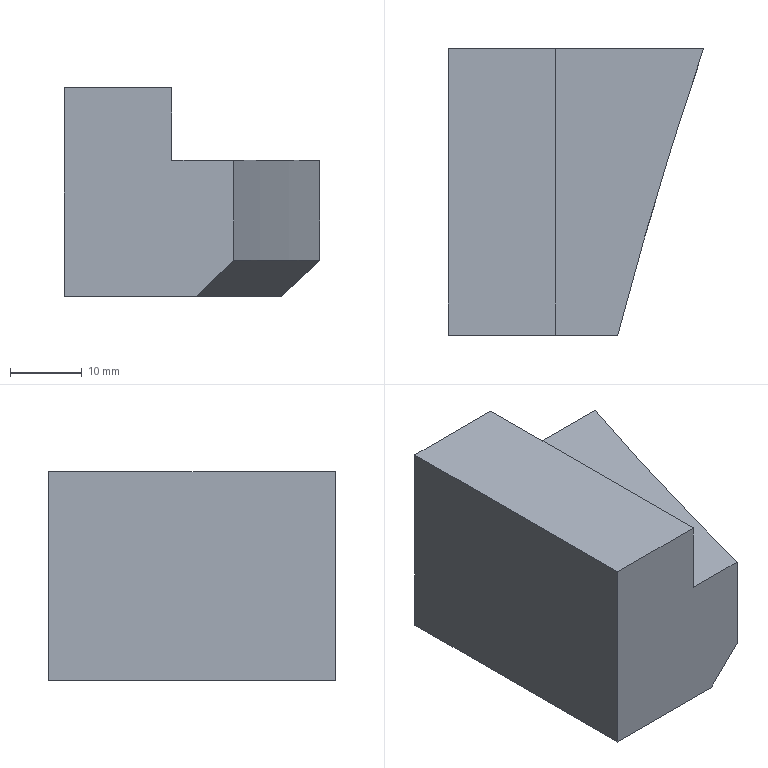Part | STEP file | Positioning_id250_x_t | 1 solid | 9 faces | box 35.628 x 40 x 29.102 mm | volume 27843 mm3 | plane 7 | spline 2
STEP:
#1=CARTESIAN_POINT('',(0.,0.,0.));
#2=DIRECTION('',(0.,0.,1.));
#3=DIRECTION('',(1.,0.,0.));
#4=AXIS2_PLACEMENT_3D('',#1,#2,#3);
#5=CARTESIAN_POINT('',(-770.37,465.,235.893));
#6=VERTEX_POINT('',#5);
#7=CARTESIAN_POINT('',(-765.202,465.,240.893));
#8=VERTEX_POINT('',#7);
#9=CARTESIAN_POINT('',(-770.37,465.,235.893));
#10=CARTESIAN_POINT('',(-769.508,465.,236.726));
#11=CARTESIAN_POINT('',(-768.647,465.,237.56));
#12=CARTESIAN_POINT('',(-767.786,465.,238.393));
#13=CARTESIAN_POINT('',(-766.924,465.,239.226));
#14=CARTESIAN_POINT('',(-766.063,465.,240.06));
#15=CARTESIAN_POINT('',(-765.202,465.,240.893));
#16=B_SPLINE_CURVE_WITH_KNOTS('',3,(#9,#10,#11,#12,#13,#14,#15),.UNSPECIFIED.,.F.,.F.,(4,3,4),(0.,0.5,1.),.UNSPECIFIED.);
#17=CARTESIAN_POINT('',(-765.482,463.728,240.943));
#18=CARTESIAN_POINT('',(-763.676,470.672,240.943));
#19=CARTESIAN_POINT('',(-759.81,484.505,240.943));
#20=CARTESIAN_POINT('',(-755.452,498.19,240.943));
#21=CARTESIAN_POINT('',(-753.154,504.984,240.943));
#22=CARTESIAN_POINT('',(-765.498,463.733,240.926));
#23=CARTESIAN_POINT('',(-763.692,470.676,240.926));
#24=CARTESIAN_POINT('',(-759.826,484.51,240.926));
#25=CARTESIAN_POINT('',(-755.468,498.195,240.926));
#26=CARTESIAN_POINT('',(-753.169,504.989,240.926));
#27=CARTESIAN_POINT('',(-765.514,463.737,240.909));
#28=CARTESIAN_POINT('',(-763.708,470.681,240.909));
#29=CARTESIAN_POINT('',(-759.842,484.515,240.909));
#30=CARTESIAN_POINT('',(-755.484,498.2,240.909));
#31=CARTESIAN_POINT('',(-753.185,504.995,240.909));
#32=CARTESIAN_POINT('',(-765.531,463.741,240.893));
#33=CARTESIAN_POINT('',(-763.724,470.685,240.893));
#34=CARTESIAN_POINT('',(-759.858,484.52,240.893));
#35=CARTESIAN_POINT('',(-755.5,498.205,240.893));
#36=CARTESIAN_POINT('',(-753.201,505.,240.893));
#37=CARTESIAN_POINT('',(-767.144,464.161,239.226));
#38=CARTESIAN_POINT('',(-765.332,471.124,239.226));
#39=CARTESIAN_POINT('',(-761.455,484.997,239.226));
#40=CARTESIAN_POINT('',(-757.085,498.72,239.226));
#41=CARTESIAN_POINT('',(-754.78,505.534,239.226));
#42=CARTESIAN_POINT('',(-768.757,464.58,237.559));
#43=CARTESIAN_POINT('',(-766.94,471.563,237.559));
#44=CARTESIAN_POINT('',(-763.052,485.474,237.559));
#45=CARTESIAN_POINT('',(-758.67,499.236,237.559));
#46=CARTESIAN_POINT('',(-756.358,506.068,237.559));
#47=CARTESIAN_POINT('',(-770.37,465.,235.893));
#48=CARTESIAN_POINT('',(-768.548,472.002,235.893));
#49=CARTESIAN_POINT('',(-764.65,485.952,235.893));
#50=CARTESIAN_POINT('',(-760.255,499.751,235.893));
#51=CARTESIAN_POINT('',(-757.937,506.602,235.893));
#52=B_SPLINE_SURFACE_WITH_KNOTS('',3,3,((#17,#18,#19,#20,#21),(#22,#23,#24,#25,#26),(#27,#28,#29,#30,#31),(#32,#33,#34,#35,#36),(#37,#38,#39,#40,#41),(#42,#43,#44,#45,#46),(#47,#48,#49,#50,#51)),.UNSPECIFIED.,.F.,.F.,.F.,(4,3,4),(4,1,4),(0.,0.009901,1.),(0.,0.5,1.),.UNSPECIFIED.);
#53=CARTESIAN_POINT('',(1.,0.));
#54=CARTESIAN_POINT('',(0.009901,0.03023));
#55=B_SPLINE_CURVE_WITH_KNOTS('',1,(#53,#54),.UNSPECIFIED.,.F.,.F.,(2,2),(0.,1.),.PIECEWISE_BEZIER_KNOTS.);
#56=(GEOMETRIC_REPRESENTATION_CONTEXT(2)PARAMETRIC_REPRESENTATION_CONTEXT()REPRESENTATION_CONTEXT('',''));
#57=DEFINITIONAL_REPRESENTATION('',(#55),#56);
#58=PCURVE('',#52,#57);
#59=CARTESIAN_POINT('',(-863.829,465.,302.856));
#60=DIRECTION('',(0.,-1.,0.));
#61=DIRECTION('',(0.,0.,1.));
#62=AXIS2_PLACEMENT_3D('',#59,#60,#61);
#63=PLANE('',#62);
#64=CARTESIAN_POINT('',(-66.963,-93.459));
#65=CARTESIAN_POINT('',(-66.13,-94.32));
#66=CARTESIAN_POINT('',(-65.296,-95.182));
#67=CARTESIAN_POINT('',(-64.463,-96.043));
#68=CARTESIAN_POINT('',(-63.63,-96.904));
#69=CARTESIAN_POINT('',(-62.796,-97.766));
#70=CARTESIAN_POINT('',(-61.963,-98.627));
#71=B_SPLINE_CURVE_WITH_KNOTS('',3,(#64,#65,#66,#67,#68,#69,#70),.UNSPECIFIED.,.F.,.F.,(4,3,4),(0.,0.5,1.),.UNSPECIFIED.);
#72=(GEOMETRIC_REPRESENTATION_CONTEXT(2)PARAMETRIC_REPRESENTATION_CONTEXT()REPRESENTATION_CONTEXT('',''));
#73=DEFINITIONAL_REPRESENTATION('',(#71),#72);
#74=PCURVE('',#63,#73);
#75=SURFACE_CURVE('',#16,(#58,#74),.PCURVE_S1.);
#76=EDGE_CURVE('',#6,#8,#75,.T.);
#77=ORIENTED_EDGE('',*,*,#76,.F.);
#78=CARTESIAN_POINT('',(-758.477,505.,235.893));
#79=VERTEX_POINT('',#78);
#80=CARTESIAN_POINT('',(-758.477,505.,235.893));
#81=CARTESIAN_POINT('',(-760.597,498.676,235.893));
#82=CARTESIAN_POINT('',(-764.802,485.408,235.893));
#83=CARTESIAN_POINT('',(-768.548,472.002,235.893));
#84=CARTESIAN_POINT('',(-770.37,465.,235.893));
#85=B_SPLINE_CURVE_WITH_KNOTS('',3,(#80,#81,#82,#83,#84),.UNSPECIFIED.,.F.,.F.,(4,1,4),(0.,0.4797,1.),.UNSPECIFIED.);
#86=CARTESIAN_POINT('',(1.,0.961));
#87=CARTESIAN_POINT('',(1.,0.));
#88=B_SPLINE_CURVE_WITH_KNOTS('',1,(#86,#87),.UNSPECIFIED.,.F.,.F.,(2,2),(0.,1.),.PIECEWISE_BEZIER_KNOTS.);
#89=(GEOMETRIC_REPRESENTATION_CONTEXT(2)PARAMETRIC_REPRESENTATION_CONTEXT()REPRESENTATION_CONTEXT('',''));
#90=DEFINITIONAL_REPRESENTATION('',(#88),#89);
#91=PCURVE('',#52,#90);
#92=CARTESIAN_POINT('',(-788.829,465.,235.893));
#93=DIRECTION('',(0.,0.,1.));
#94=DIRECTION('',(1.,0.,0.));
#95=AXIS2_PLACEMENT_3D('',#92,#93,#94);
#96=PLANE('',#95);
#97=CARTESIAN_POINT('',(30.352,40.));
#98=CARTESIAN_POINT('',(28.232,33.675));
#99=CARTESIAN_POINT('',(24.027,20.408));
#100=CARTESIAN_POINT('',(20.281,7.002));
#101=CARTESIAN_POINT('',(18.459,-0.000000011));
#102=B_SPLINE_CURVE_WITH_KNOTS('',3,(#97,#98,#99,#100,#101),.UNSPECIFIED.,.F.,.F.,(4,1,4),(0.,0.4797,1.),.UNSPECIFIED.);
#103=(GEOMETRIC_REPRESENTATION_CONTEXT(2)PARAMETRIC_REPRESENTATION_CONTEXT()REPRESENTATION_CONTEXT('',''));
#104=DEFINITIONAL_REPRESENTATION('',(#102),#103);
#105=PCURVE('',#96,#104);
#106=SURFACE_CURVE('',#85,(#91,#105),.PCURVE_S1.);
#107=EDGE_CURVE('',#79,#6,#106,.T.);
#108=ORIENTED_EDGE('',*,*,#107,.F.);
#109=CARTESIAN_POINT('',(-753.201,505.,240.893));
#110=VERTEX_POINT('',#109);
#111=CARTESIAN_POINT('',(-753.201,505.,240.893));
#112=CARTESIAN_POINT('',(-754.08,505.,240.06));
#113=CARTESIAN_POINT('',(-754.96,505.,239.226));
#114=CARTESIAN_POINT('',(-755.839,505.,238.393));
#115=CARTESIAN_POINT('',(-756.718,505.,237.56));
#116=CARTESIAN_POINT('',(-757.598,505.,236.726));
#117=CARTESIAN_POINT('',(-758.477,505.,235.893));
#118=B_SPLINE_CURVE_WITH_KNOTS('',3,(#111,#112,#113,#114,#115,#116,#117),.UNSPECIFIED.,.F.,.F.,(4,3,4),(0.,0.5,1.),.UNSPECIFIED.);
#119=CARTESIAN_POINT('',(0.009906,1.));
#120=CARTESIAN_POINT('',(1.,0.961));
#121=B_SPLINE_CURVE_WITH_KNOTS('',1,(#119,#120),.UNSPECIFIED.,.F.,.F.,(2,2),(0.,1.),.PIECEWISE_BEZIER_KNOTS.);
#122=(GEOMETRIC_REPRESENTATION_CONTEXT(2)PARAMETRIC_REPRESENTATION_CONTEXT()REPRESENTATION_CONTEXT('',''));
#123=DEFINITIONAL_REPRESENTATION('',(#121),#122);
#124=PCURVE('',#52,#123);
#125=CARTESIAN_POINT('',(-863.829,505.,302.856));
#126=DIRECTION('',(0.,1.,0.));
#127=DIRECTION('',(0.,0.,-1.));
#128=AXIS2_PLACEMENT_3D('',#125,#126,#127);
#129=PLANE('',#128);
#130=CARTESIAN_POINT('',(61.963,-110.628));
#131=CARTESIAN_POINT('',(62.796,-109.748));
#132=CARTESIAN_POINT('',(63.629,-108.869));
#133=CARTESIAN_POINT('',(64.463,-107.99));
#134=CARTESIAN_POINT('',(65.296,-107.11));
#135=CARTESIAN_POINT('',(66.13,-106.231));
#136=CARTESIAN_POINT('',(66.963,-105.352));
#137=B_SPLINE_CURVE_WITH_KNOTS('',3,(#130,#131,#132,#133,#134,#135,#136),.UNSPECIFIED.,.F.,.F.,(4,3,4),(0.,0.5,1.),.UNSPECIFIED.);
#138=(GEOMETRIC_REPRESENTATION_CONTEXT(2)PARAMETRIC_REPRESENTATION_CONTEXT()REPRESENTATION_CONTEXT('',''));
#139=DEFINITIONAL_REPRESENTATION('',(#137),#138);
#140=PCURVE('',#129,#139);
#141=SURFACE_CURVE('',#118,(#124,#140),.PCURVE_S1.);
#142=EDGE_CURVE('',#110,#79,#141,.T.);
#143=ORIENTED_EDGE('',*,*,#142,.F.);
#144=CARTESIAN_POINT('',(-765.202,465.,240.893));
#145=CARTESIAN_POINT('',(-764.004,469.56,240.893));
#146=CARTESIAN_POINT('',(-762.753,474.107,240.893));
#147=CARTESIAN_POINT('',(-761.449,478.638,240.893));
#148=CARTESIAN_POINT('',(-760.176,483.061,240.893));
#149=CARTESIAN_POINT('',(-758.852,487.47,240.893));
#150=CARTESIAN_POINT('',(-757.478,491.863,240.893));
#151=CARTESIAN_POINT('',(-756.102,496.258,240.893));
#152=CARTESIAN_POINT('',(-754.677,500.638,240.893));
#153=CARTESIAN_POINT('',(-753.201,505.,240.893));
#154=B_SPLINE_CURVE_WITH_KNOTS('',3,(#144,#145,#146,#147,#148,#149,#150,#151,#152,#153),.UNSPECIFIED.,.F.,.F.,(4,3,3,4),(0.,0.3386,0.6692,1.),.UNSPECIFIED.);
#155=CARTESIAN_POINT('',(0.009894,0.03023));
#156=CARTESIAN_POINT('',(0.009903,1.));
#157=B_SPLINE_CURVE_WITH_KNOTS('',1,(#155,#156),.UNSPECIFIED.,.F.,.F.,(2,2),(0.,1.),.PIECEWISE_BEZIER_KNOTS.);
#158=(GEOMETRIC_REPRESENTATION_CONTEXT(2)PARAMETRIC_REPRESENTATION_CONTEXT()REPRESENTATION_CONTEXT('',''));
#159=DEFINITIONAL_REPRESENTATION('',(#157),#158);
#160=PCURVE('',#52,#159);
#161=CARTESIAN_POINT('',(-753.201,505.,240.753));
#162=CARTESIAN_POINT('',(-753.201,505.,240.893));
#163=CARTESIAN_POINT('',(-753.201,505.,254.856));
#164=CARTESIAN_POINT('',(-757.663,491.811,240.753));
#165=CARTESIAN_POINT('',(-757.663,491.811,240.893));
#166=CARTESIAN_POINT('',(-757.663,491.811,254.856));
#167=CARTESIAN_POINT('',(-761.665,478.472,240.753));
#168=CARTESIAN_POINT('',(-761.665,478.472,240.893));
#169=CARTESIAN_POINT('',(-761.665,478.472,254.856));
#170=CARTESIAN_POINT('',(-765.202,465.,240.753));
#171=CARTESIAN_POINT('',(-765.202,465.,240.893));
#172=CARTESIAN_POINT('',(-765.202,465.,254.856));
#173=CARTESIAN_POINT('',(-765.237,464.865,240.753));
#174=CARTESIAN_POINT('',(-765.237,464.865,240.893));
#175=CARTESIAN_POINT('',(-765.237,464.865,254.856));
#176=CARTESIAN_POINT('',(-765.272,464.731,240.753));
#177=CARTESIAN_POINT('',(-765.272,464.731,240.893));
#178=CARTESIAN_POINT('',(-765.272,464.731,254.856));
#179=CARTESIAN_POINT('',(-765.308,464.596,240.753));
#180=CARTESIAN_POINT('',(-765.308,464.596,240.893));
#181=CARTESIAN_POINT('',(-765.308,464.596,254.856));
#182=(BOUNDED_SURFACE()B_SPLINE_SURFACE(3,1,((#161,#162,#163),(#164,#165,#166),(#167,#168,#169),(#170,#171,#172),(#173,#174,#175),(#176,#177,#178),(#179,#180,#181)),.UNSPECIFIED.,.F.,.F.,.F.)B_SPLINE_SURFACE_WITH_KNOTS((4,3,4),(2,1,2),(0.,0.9901,1.),(0.,0.009901,1.),.UNSPECIFIED.)GEOMETRIC_REPRESENTATION_ITEM()RATIONAL_B_SPLINE_SURFACE(((0.9919,0.9919,0.9919),(0.9912,0.9912,0.9912),(0.9909,0.9909,0.9909),(0.9909,0.9909,0.9909),(0.9909,0.9909,0.9909),(0.9909,0.9909,0.9909),(0.9909,0.9909,0.9909)))REPRESENTATION_ITEM('')SURFACE());
#183=CARTESIAN_POINT('',(0.9901,0.009906));
#184=CARTESIAN_POINT('',(0.,0.009903));
#185=B_SPLINE_CURVE_WITH_KNOTS('',1,(#183,#184),.UNSPECIFIED.,.F.,.F.,(2,2),(0.,1.),.PIECEWISE_BEZIER_KNOTS.);
#186=(GEOMETRIC_REPRESENTATION_CONTEXT(2)PARAMETRIC_REPRESENTATION_CONTEXT()REPRESENTATION_CONTEXT('',''));
#187=DEFINITIONAL_REPRESENTATION('',(#185),#186);
#188=PCURVE('',#182,#187);
#189=SURFACE_CURVE('',#154,(#160,#188),.PCURVE_S1.);
#190=EDGE_CURVE('',#8,#110,#189,.T.);
#191=ORIENTED_EDGE('',*,*,#190,.F.);
#192=EDGE_LOOP('',(#77,#108,#143,#191));
#193=FACE_BOUND('',#192,.T.);
#194=ADVANCED_FACE('',(#193),#52,.T.);
#195=CARTESIAN_POINT('',(-788.829,465.,235.893));
#196=VERTEX_POINT('',#195);
#197=CARTESIAN_POINT('',(-788.829,505.,235.893));
#198=VERTEX_POINT('',#197);
#199=CARTESIAN_POINT('',(-788.829,465.,235.893));
#200=DIRECTION('',(0.,1.,0.));
#201=VECTOR('',#200,1.);
#202=LINE('',#199,#201);
#203=CARTESIAN_POINT('',(0.,0.));
#204=DIRECTION('',(0.,1.));
#205=VECTOR('',#204,1.);
#206=LINE('',#203,#205);
#207=(GEOMETRIC_REPRESENTATION_CONTEXT(2)PARAMETRIC_REPRESENTATION_CONTEXT()REPRESENTATION_CONTEXT('',''));
#208=DEFINITIONAL_REPRESENTATION('',(#206),#207);
#209=PCURVE('',#96,#208);
#210=CARTESIAN_POINT('',(-788.829,493.037,302.856));
#211=DIRECTION('',(-1.,0.,0.));
#212=DIRECTION('',(0.,0.,1.));
#213=AXIS2_PLACEMENT_3D('',#210,#211,#212);
#214=PLANE('',#213);
#215=CARTESIAN_POINT('',(-66.963,-28.037));
#216=DIRECTION('',(0.,1.));
#217=VECTOR('',#216,1.);
#218=LINE('',#215,#217);
#219=(GEOMETRIC_REPRESENTATION_CONTEXT(2)PARAMETRIC_REPRESENTATION_CONTEXT()REPRESENTATION_CONTEXT('',''));
#220=DEFINITIONAL_REPRESENTATION('',(#218),#219);
#221=PCURVE('',#214,#220);
#222=SURFACE_CURVE('',#202,(#209,#221),.PCURVE_S1.);
#223=EDGE_CURVE('',#196,#198,#222,.T.);
#224=ORIENTED_EDGE('',*,*,#223,.F.);
#225=CARTESIAN_POINT('',(-770.37,465.,235.893));
#226=DIRECTION('',(-1.,0.,0.));
#227=VECTOR('',#226,1.);
#228=LINE('',#225,#227);
#229=CARTESIAN_POINT('',(18.459,0.));
#230=DIRECTION('',(-1.,0.));
#231=VECTOR('',#230,1.);
#232=LINE('',#229,#231);
#233=(GEOMETRIC_REPRESENTATION_CONTEXT(2)PARAMETRIC_REPRESENTATION_CONTEXT()REPRESENTATION_CONTEXT('',''));
#234=DEFINITIONAL_REPRESENTATION('',(#232),#233);
#235=PCURVE('',#96,#234);
#236=CARTESIAN_POINT('',(-66.963,-93.459));
#237=DIRECTION('',(0.,1.));
#238=VECTOR('',#237,1.);
#239=LINE('',#236,#238);
#240=(GEOMETRIC_REPRESENTATION_CONTEXT(2)PARAMETRIC_REPRESENTATION_CONTEXT()REPRESENTATION_CONTEXT('',''));
#241=DEFINITIONAL_REPRESENTATION('',(#239),#240);
#242=PCURVE('',#63,#241);
#243=SURFACE_CURVE('',#228,(#235,#242),.PCURVE_S1.);
#244=EDGE_CURVE('',#6,#196,#243,.T.);
#245=ORIENTED_EDGE('',*,*,#244,.F.);
#246=ORIENTED_EDGE('',*,*,#107,.F.);
#247=CARTESIAN_POINT('',(-788.829,505.,235.893));
#248=DIRECTION('',(1.,0.,0.));
#249=VECTOR('',#248,1.);
#250=LINE('',#247,#249);
#251=CARTESIAN_POINT('',(0.,40.));
#252=DIRECTION('',(1.,0.));
#253=VECTOR('',#252,1.);
#254=LINE('',#251,#253);
#255=(GEOMETRIC_REPRESENTATION_CONTEXT(2)PARAMETRIC_REPRESENTATION_CONTEXT()REPRESENTATION_CONTEXT('',''));
#256=DEFINITIONAL_REPRESENTATION('',(#254),#255);
#257=PCURVE('',#96,#256);
#258=CARTESIAN_POINT('',(66.963,-75.));
#259=DIRECTION('',(0.,-1.));
#260=VECTOR('',#259,1.);
#261=LINE('',#258,#260);
#262=(GEOMETRIC_REPRESENTATION_CONTEXT(2)PARAMETRIC_REPRESENTATION_CONTEXT()REPRESENTATION_CONTEXT('',''));
#263=DEFINITIONAL_REPRESENTATION('',(#261),#262);
#264=PCURVE('',#129,#263);
#265=SURFACE_CURVE('',#250,(#257,#264),.PCURVE_S1.);
#266=EDGE_CURVE('',#198,#79,#265,.T.);
#267=ORIENTED_EDGE('',*,*,#266,.F.);
#268=EDGE_LOOP('',(#224,#245,#246,#267));
#269=FACE_BOUND('',#268,.F.);
#270=ADVANCED_FACE('',(#269),#96,.F.);
#271=CARTESIAN_POINT('',(-753.201,505.,254.856));
#272=VERTEX_POINT('',#271);
#273=CARTESIAN_POINT('',(-765.202,465.,254.856));
#274=VERTEX_POINT('',#273);
#275=CARTESIAN_POINT('',(-753.201,505.,254.856));
#276=CARTESIAN_POINT('',(-757.663,491.811,254.856));
#277=CARTESIAN_POINT('',(-761.665,478.472,254.856));
#278=CARTESIAN_POINT('',(-765.202,465.,254.856));
#279=(BOUNDED_CURVE()B_SPLINE_CURVE(3,(#275,#276,#277,#278),.UNSPECIFIED.,.F.,.F.)B_SPLINE_CURVE_WITH_KNOTS((4,4),(0.,1.),.PIECEWISE_BEZIER_KNOTS.)CURVE()GEOMETRIC_REPRESENTATION_ITEM()RATIONAL_B_SPLINE_CURVE((0.9919,0.9912,0.9909,0.9909))REPRESENTATION_ITEM(''));
#280=CARTESIAN_POINT('',(0.,1.));
#281=CARTESIAN_POINT('',(0.9901,1.));
#282=B_SPLINE_CURVE_WITH_KNOTS('',1,(#280,#281),.UNSPECIFIED.,.F.,.F.,(2,2),(0.,1.),.PIECEWISE_BEZIER_KNOTS.);
#283=(GEOMETRIC_REPRESENTATION_CONTEXT(2)PARAMETRIC_REPRESENTATION_CONTEXT()REPRESENTATION_CONTEXT('',''));
#284=DEFINITIONAL_REPRESENTATION('',(#282),#283);
#285=PCURVE('',#182,#284);
#286=CARTESIAN_POINT('',(-853.829,493.037,254.856));
#287=DIRECTION('',(0.,0.,1.));
#288=DIRECTION('',(1.,0.,0.));
#289=AXIS2_PLACEMENT_3D('',#286,#287,#288);
#290=PLANE('',#289);
#291=CARTESIAN_POINT('',(100.628,11.963));
#292=CARTESIAN_POINT('',(96.166,-1.226));
#293=CARTESIAN_POINT('',(92.164,-14.565));
#294=CARTESIAN_POINT('',(88.627,-28.037));
#295=(BOUNDED_CURVE()B_SPLINE_CURVE(3,(#291,#292,#293,#294),.UNSPECIFIED.,.F.,.F.)B_SPLINE_CURVE_WITH_KNOTS((4,4),(0.,1.),.PIECEWISE_BEZIER_KNOTS.)CURVE()GEOMETRIC_REPRESENTATION_ITEM()RATIONAL_B_SPLINE_CURVE((0.9919,0.9912,0.9909,0.9909))REPRESENTATION_ITEM(''));
#296=(GEOMETRIC_REPRESENTATION_CONTEXT(2)PARAMETRIC_REPRESENTATION_CONTEXT()REPRESENTATION_CONTEXT('',''));
#297=DEFINITIONAL_REPRESENTATION('',(#295),#296);
#298=PCURVE('',#290,#297);
#299=SURFACE_CURVE('',#279,(#285,#298),.PCURVE_S1.);
#300=EDGE_CURVE('',#272,#274,#299,.T.);
#301=ORIENTED_EDGE('',*,*,#300,.F.);
#302=CARTESIAN_POINT('',(-753.201,505.,240.893));
#303=DIRECTION('',(0.,0.,1.));
#304=VECTOR('',#303,1.);
#305=LINE('',#302,#304);
#306=CARTESIAN_POINT('',(0.,0.009901));
#307=CARTESIAN_POINT('',(0.,1.));
#308=B_SPLINE_CURVE_WITH_KNOTS('',1,(#306,#307),.UNSPECIFIED.,.F.,.F.,(2,2),(0.,13.963),.PIECEWISE_BEZIER_KNOTS.);
#309=(GEOMETRIC_REPRESENTATION_CONTEXT(2)PARAMETRIC_REPRESENTATION_CONTEXT()REPRESENTATION_CONTEXT('',''));
#310=DEFINITIONAL_REPRESENTATION('',(#308),#309);
#311=PCURVE('',#182,#310);
#312=CARTESIAN_POINT('',(61.963,-110.628));
#313=DIRECTION('',(-1.,0.));
#314=VECTOR('',#313,1.);
#315=LINE('',#312,#314);
#316=(GEOMETRIC_REPRESENTATION_CONTEXT(2)PARAMETRIC_REPRESENTATION_CONTEXT()REPRESENTATION_CONTEXT('',''));
#317=DEFINITIONAL_REPRESENTATION('',(#315),#316);
#318=PCURVE('',#129,#317);
#319=SURFACE_CURVE('',#305,(#311,#318),.PCURVE_S1.);
#320=EDGE_CURVE('',#110,#272,#319,.T.);
#321=ORIENTED_EDGE('',*,*,#320,.F.);
#322=ORIENTED_EDGE('',*,*,#190,.F.);
#323=CARTESIAN_POINT('',(-765.202,465.,254.856));
#324=DIRECTION('',(0.,0.,-1.));
#325=VECTOR('',#324,1.);
#326=LINE('',#323,#325);
#327=CARTESIAN_POINT('',(0.9901,1.));
#328=CARTESIAN_POINT('',(0.9901,0.009904));
#329=B_SPLINE_CURVE_WITH_KNOTS('',1,(#327,#328),.UNSPECIFIED.,.F.,.F.,(2,2),(0.,13.963),.PIECEWISE_BEZIER_KNOTS.);
#330=(GEOMETRIC_REPRESENTATION_CONTEXT(2)PARAMETRIC_REPRESENTATION_CONTEXT()REPRESENTATION_CONTEXT('',''));
#331=DEFINITIONAL_REPRESENTATION('',(#329),#330);
#332=PCURVE('',#182,#331);
#333=CARTESIAN_POINT('',(-48.,-98.627));
#334=DIRECTION('',(-1.,0.));
#335=VECTOR('',#334,1.);
#336=LINE('',#333,#335);
#337=(GEOMETRIC_REPRESENTATION_CONTEXT(2)PARAMETRIC_REPRESENTATION_CONTEXT()REPRESENTATION_CONTEXT('',''));
#338=DEFINITIONAL_REPRESENTATION('',(#336),#337);
#339=PCURVE('',#63,#338);
#340=SURFACE_CURVE('',#326,(#332,#339),.PCURVE_S1.);
#341=EDGE_CURVE('',#274,#8,#340,.T.);
#342=ORIENTED_EDGE('',*,*,#341,.F.);
#343=EDGE_LOOP('',(#301,#321,#322,#342));
#344=FACE_BOUND('',#343,.F.);
#345=ADVANCED_FACE('',(#344),#182,.F.);
#346=ORIENTED_EDGE('',*,*,#300,.F.);
#347=CARTESIAN_POINT('',(-773.829,505.,254.856));
#348=VERTEX_POINT('',#347);
#349=CARTESIAN_POINT('',(-773.829,505.,254.856));
#350=DIRECTION('',(1.,0.,0.));
#351=VECTOR('',#350,1.);
#352=LINE('',#349,#351);
#353=CARTESIAN_POINT('',(80.,11.963));
#354=DIRECTION('',(1.,0.));
#355=VECTOR('',#354,1.);
#356=LINE('',#353,#355);
#357=(GEOMETRIC_REPRESENTATION_CONTEXT(2)PARAMETRIC_REPRESENTATION_CONTEXT()REPRESENTATION_CONTEXT('',''));
#358=DEFINITIONAL_REPRESENTATION('',(#356),#357);
#359=PCURVE('',#290,#358);
#360=CARTESIAN_POINT('',(48.,-90.));
#361=DIRECTION('',(0.,-1.));
#362=VECTOR('',#361,1.);
#363=LINE('',#360,#362);
#364=(GEOMETRIC_REPRESENTATION_CONTEXT(2)PARAMETRIC_REPRESENTATION_CONTEXT()REPRESENTATION_CONTEXT('',''));
#365=DEFINITIONAL_REPRESENTATION('',(#363),#364);
#366=PCURVE('',#129,#365);
#367=SURFACE_CURVE('',#352,(#359,#366),.PCURVE_S1.);
#368=EDGE_CURVE('',#348,#272,#367,.T.);
#369=ORIENTED_EDGE('',*,*,#368,.F.);
#370=CARTESIAN_POINT('',(-773.829,465.,254.856));
#371=VERTEX_POINT('',#370);
#372=CARTESIAN_POINT('',(-773.829,505.,254.856));
#373=DIRECTION('',(0.,-1.,0.));
#374=VECTOR('',#373,1.);
#375=LINE('',#372,#374);
#376=CARTESIAN_POINT('',(80.,11.963));
#377=DIRECTION('',(0.,-1.));
#378=VECTOR('',#377,1.);
#379=LINE('',#376,#378);
#380=(GEOMETRIC_REPRESENTATION_CONTEXT(2)PARAMETRIC_REPRESENTATION_CONTEXT()REPRESENTATION_CONTEXT('',''));
#381=DEFINITIONAL_REPRESENTATION('',(#379),#380);
#382=PCURVE('',#290,#381);
#383=CARTESIAN_POINT('',(-773.829,463.037,251.856));
#384=DIRECTION('',(1.,0.,0.));
#385=DIRECTION('',(0.,0.,-1.));
#386=AXIS2_PLACEMENT_3D('',#383,#384,#385);
#387=PLANE('',#386);
#388=CARTESIAN_POINT('',(-3.,41.963));
#389=DIRECTION('',(0.,-1.));
#390=VECTOR('',#389,1.);
#391=LINE('',#388,#390);
#392=(GEOMETRIC_REPRESENTATION_CONTEXT(2)PARAMETRIC_REPRESENTATION_CONTEXT()REPRESENTATION_CONTEXT('',''));
#393=DEFINITIONAL_REPRESENTATION('',(#391),#392);
#394=PCURVE('',#387,#393);
#395=SURFACE_CURVE('',#375,(#382,#394),.PCURVE_S1.);
#396=EDGE_CURVE('',#348,#371,#395,.T.);
#397=ORIENTED_EDGE('',*,*,#396,.T.);
#398=CARTESIAN_POINT('',(-765.202,465.,254.856));
#399=DIRECTION('',(-1.,0.,0.));
#400=VECTOR('',#399,1.);
#401=LINE('',#398,#400);
#402=CARTESIAN_POINT('',(88.627,-28.037));
#403=DIRECTION('',(-1.,0.));
#404=VECTOR('',#403,1.);
#405=LINE('',#402,#404);
#406=(GEOMETRIC_REPRESENTATION_CONTEXT(2)PARAMETRIC_REPRESENTATION_CONTEXT()REPRESENTATION_CONTEXT('',''));
#407=DEFINITIONAL_REPRESENTATION('',(#405),#406);
#408=PCURVE('',#290,#407);
#409=CARTESIAN_POINT('',(-48.,-98.627));
#410=DIRECTION('',(0.,1.));
#411=VECTOR('',#410,1.);
#412=LINE('',#409,#411);
#413=(GEOMETRIC_REPRESENTATION_CONTEXT(2)PARAMETRIC_REPRESENTATION_CONTEXT()REPRESENTATION_CONTEXT('',''));
#414=DEFINITIONAL_REPRESENTATION('',(#412),#413);
#415=PCURVE('',#63,#414);
#416=SURFACE_CURVE('',#401,(#408,#415),.PCURVE_S1.);
#417=EDGE_CURVE('',#274,#371,#416,.T.);
#418=ORIENTED_EDGE('',*,*,#417,.F.);
#419=EDGE_LOOP('',(#346,#369,#397,#418));
#420=FACE_BOUND('',#419,.T.);
#421=ADVANCED_FACE('',(#420),#290,.T.);
#422=CARTESIAN_POINT('',(-788.829,465.,264.995));
#423=VERTEX_POINT('',#422);
#424=CARTESIAN_POINT('',(-788.829,465.,264.995));
#425=DIRECTION('',(0.,0.,-1.));
#426=VECTOR('',#425,1.);
#427=LINE('',#424,#426);
#428=CARTESIAN_POINT('',(-37.861,-28.037));
#429=DIRECTION('',(-1.,0.));
#430=VECTOR('',#429,1.);
#431=LINE('',#428,#430);
#432=(GEOMETRIC_REPRESENTATION_CONTEXT(2)PARAMETRIC_REPRESENTATION_CONTEXT()REPRESENTATION_CONTEXT('',''));
#433=DEFINITIONAL_REPRESENTATION('',(#431),#432);
#434=PCURVE('',#214,#433);
#435=CARTESIAN_POINT('',(-37.861,-75.));
#436=DIRECTION('',(-1.,0.));
#437=VECTOR('',#436,1.);
#438=LINE('',#435,#437);
#439=(GEOMETRIC_REPRESENTATION_CONTEXT(2)PARAMETRIC_REPRESENTATION_CONTEXT()REPRESENTATION_CONTEXT('',''));
#440=DEFINITIONAL_REPRESENTATION('',(#438),#439);
#441=PCURVE('',#63,#440);
#442=SURFACE_CURVE('',#427,(#434,#441),.PCURVE_S1.);
#443=EDGE_CURVE('',#423,#196,#442,.T.);
#444=ORIENTED_EDGE('',*,*,#443,.F.);
#445=CARTESIAN_POINT('',(-788.829,505.,264.995));
#446=VERTEX_POINT('',#445);
#447=CARTESIAN_POINT('',(-788.829,505.,264.995));
#448=DIRECTION('',(0.,-1.,0.));
#449=VECTOR('',#448,1.);
#450=LINE('',#447,#449);
#451=CARTESIAN_POINT('',(-37.861,11.963));
#452=DIRECTION('',(0.,-1.));
#453=VECTOR('',#452,1.);
#454=LINE('',#451,#453);
#455=(GEOMETRIC_REPRESENTATION_CONTEXT(2)PARAMETRIC_REPRESENTATION_CONTEXT()REPRESENTATION_CONTEXT('',''));
#456=DEFINITIONAL_REPRESENTATION('',(#454),#455);
#457=PCURVE('',#214,#456);
#458=CARTESIAN_POINT('',(-843.829,463.037,264.995));
#459=DIRECTION('',(0.,0.,-1.));
#460=DIRECTION('',(-1.,0.,0.));
#461=AXIS2_PLACEMENT_3D('',#458,#459,#460);
#462=PLANE('',#461);
#463=CARTESIAN_POINT('',(-55.,41.963));
#464=DIRECTION('',(0.,-1.));
#465=VECTOR('',#464,1.);
#466=LINE('',#463,#465);
#467=(GEOMETRIC_REPRESENTATION_CONTEXT(2)PARAMETRIC_REPRESENTATION_CONTEXT()REPRESENTATION_CONTEXT('',''));
#468=DEFINITIONAL_REPRESENTATION('',(#466),#467);
#469=PCURVE('',#462,#468);
#470=SURFACE_CURVE('',#450,(#457,#469),.PCURVE_S1.);
#471=EDGE_CURVE('',#446,#423,#470,.T.);
#472=ORIENTED_EDGE('',*,*,#471,.F.);
#473=CARTESIAN_POINT('',(-788.829,505.,235.893));
#474=DIRECTION('',(0.,0.,1.));
#475=VECTOR('',#474,1.);
#476=LINE('',#473,#475);
#477=CARTESIAN_POINT('',(-66.963,11.963));
#478=DIRECTION('',(1.,0.));
#479=VECTOR('',#478,1.);
#480=LINE('',#477,#479);
#481=(GEOMETRIC_REPRESENTATION_CONTEXT(2)PARAMETRIC_REPRESENTATION_CONTEXT()REPRESENTATION_CONTEXT('',''));
#482=DEFINITIONAL_REPRESENTATION('',(#480),#481);
#483=PCURVE('',#214,#482);
#484=CARTESIAN_POINT('',(66.963,-75.));
#485=DIRECTION('',(-1.,0.));
#486=VECTOR('',#485,1.);
#487=LINE('',#484,#486);
#488=(GEOMETRIC_REPRESENTATION_CONTEXT(2)PARAMETRIC_REPRESENTATION_CONTEXT()REPRESENTATION_CONTEXT('',''));
#489=DEFINITIONAL_REPRESENTATION('',(#487),#488);
#490=PCURVE('',#129,#489);
#491=SURFACE_CURVE('',#476,(#483,#490),.PCURVE_S1.);
#492=EDGE_CURVE('',#198,#446,#491,.T.);
#493=ORIENTED_EDGE('',*,*,#492,.F.);
#494=ORIENTED_EDGE('',*,*,#223,.F.);
#495=EDGE_LOOP('',(#444,#472,#493,#494));
#496=FACE_BOUND('',#495,.T.);
#497=ADVANCED_FACE('',(#496),#214,.T.);
#498=ORIENTED_EDGE('',*,*,#396,.F.);
#499=CARTESIAN_POINT('',(-773.829,505.,264.995));
#500=VERTEX_POINT('',#499);
#501=CARTESIAN_POINT('',(-773.829,505.,264.995));
#502=DIRECTION('',(0.,0.,-1.));
#503=VECTOR('',#502,1.);
#504=LINE('',#501,#503);
#505=CARTESIAN_POINT('',(-13.139,41.963));
#506=DIRECTION('',(1.,0.));
#507=VECTOR('',#506,1.);
#508=LINE('',#505,#507);
#509=(GEOMETRIC_REPRESENTATION_CONTEXT(2)PARAMETRIC_REPRESENTATION_CONTEXT()REPRESENTATION_CONTEXT('',''));
#510=DEFINITIONAL_REPRESENTATION('',(#508),#509);
#511=PCURVE('',#387,#510);
#512=CARTESIAN_POINT('',(37.861,-90.));
#513=DIRECTION('',(1.,0.));
#514=VECTOR('',#513,1.);
#515=LINE('',#512,#514);
#516=(GEOMETRIC_REPRESENTATION_CONTEXT(2)PARAMETRIC_REPRESENTATION_CONTEXT()REPRESENTATION_CONTEXT('',''));
#517=DEFINITIONAL_REPRESENTATION('',(#515),#516);
#518=PCURVE('',#129,#517);
#519=SURFACE_CURVE('',#504,(#511,#518),.PCURVE_S1.);
#520=EDGE_CURVE('',#500,#348,#519,.T.);
#521=ORIENTED_EDGE('',*,*,#520,.F.);
#522=CARTESIAN_POINT('',(-773.829,465.,264.995));
#523=VERTEX_POINT('',#522);
#524=CARTESIAN_POINT('',(-773.829,465.,264.995));
#525=DIRECTION('',(0.,1.,0.));
#526=VECTOR('',#525,1.);
#527=LINE('',#524,#526);
#528=CARTESIAN_POINT('',(-13.139,1.963));
#529=DIRECTION('',(0.,1.));
#530=VECTOR('',#529,1.);
#531=LINE('',#528,#530);
#532=(GEOMETRIC_REPRESENTATION_CONTEXT(2)PARAMETRIC_REPRESENTATION_CONTEXT()REPRESENTATION_CONTEXT('',''));
#533=DEFINITIONAL_REPRESENTATION('',(#531),#532);
#534=PCURVE('',#387,#533);
#535=CARTESIAN_POINT('',(-70.,1.963));
#536=DIRECTION('',(0.,1.));
#537=VECTOR('',#536,1.);
#538=LINE('',#535,#537);
#539=(GEOMETRIC_REPRESENTATION_CONTEXT(2)PARAMETRIC_REPRESENTATION_CONTEXT()REPRESENTATION_CONTEXT('',''));
#540=DEFINITIONAL_REPRESENTATION('',(#538),#539);
#541=PCURVE('',#462,#540);
#542=SURFACE_CURVE('',#527,(#534,#541),.PCURVE_S1.);
#543=EDGE_CURVE('',#523,#500,#542,.T.);
#544=ORIENTED_EDGE('',*,*,#543,.F.);
#545=CARTESIAN_POINT('',(-773.829,465.,254.856));
#546=DIRECTION('',(0.,0.,1.));
#547=VECTOR('',#546,1.);
#548=LINE('',#545,#547);
#549=CARTESIAN_POINT('',(-3.,1.963));
#550=DIRECTION('',(-1.,0.));
#551=VECTOR('',#550,1.);
#552=LINE('',#549,#551);
#553=(GEOMETRIC_REPRESENTATION_CONTEXT(2)PARAMETRIC_REPRESENTATION_CONTEXT()REPRESENTATION_CONTEXT('',''));
#554=DEFINITIONAL_REPRESENTATION('',(#552),#553);
#555=PCURVE('',#387,#554);
#556=CARTESIAN_POINT('',(-48.,-90.));
#557=DIRECTION('',(1.,0.));
#558=VECTOR('',#557,1.);
#559=LINE('',#556,#558);
#560=(GEOMETRIC_REPRESENTATION_CONTEXT(2)PARAMETRIC_REPRESENTATION_CONTEXT()REPRESENTATION_CONTEXT('',''));
#561=DEFINITIONAL_REPRESENTATION('',(#559),#560);
#562=PCURVE('',#63,#561);
#563=SURFACE_CURVE('',#548,(#555,#562),.PCURVE_S1.);
#564=EDGE_CURVE('',#371,#523,#563,.T.);
#565=ORIENTED_EDGE('',*,*,#564,.F.);
#566=EDGE_LOOP('',(#498,#521,#544,#565));
#567=FACE_BOUND('',#566,.T.);
#568=ADVANCED_FACE('',(#567),#387,.T.);
#569=ORIENTED_EDGE('',*,*,#492,.T.);
#570=CARTESIAN_POINT('',(-773.829,505.,264.995));
#571=DIRECTION('',(-1.,0.,0.));
#572=VECTOR('',#571,1.);
#573=LINE('',#570,#572);
#574=CARTESIAN_POINT('',(37.861,-90.));
#575=DIRECTION('',(0.,1.));
#576=VECTOR('',#575,1.);
#577=LINE('',#574,#576);
#578=(GEOMETRIC_REPRESENTATION_CONTEXT(2)PARAMETRIC_REPRESENTATION_CONTEXT()REPRESENTATION_CONTEXT('',''));
#579=DEFINITIONAL_REPRESENTATION('',(#577),#578);
#580=PCURVE('',#129,#579);
#581=CARTESIAN_POINT('',(-70.,41.963));
#582=DIRECTION('',(1.,0.));
#583=VECTOR('',#582,1.);
#584=LINE('',#581,#583);
#585=(GEOMETRIC_REPRESENTATION_CONTEXT(2)PARAMETRIC_REPRESENTATION_CONTEXT()REPRESENTATION_CONTEXT('',''));
#586=DEFINITIONAL_REPRESENTATION('',(#584),#585);
#587=PCURVE('',#462,#586);
#588=SURFACE_CURVE('',#573,(#580,#587),.PCURVE_S1.);
#589=EDGE_CURVE('',#500,#446,#588,.T.);
#590=ORIENTED_EDGE('',*,*,#589,.F.);
#591=ORIENTED_EDGE('',*,*,#520,.T.);
#592=ORIENTED_EDGE('',*,*,#368,.T.);
#593=ORIENTED_EDGE('',*,*,#320,.F.);
#594=ORIENTED_EDGE('',*,*,#142,.T.);
#595=ORIENTED_EDGE('',*,*,#266,.F.);
#596=EDGE_LOOP('',(#569,#590,#591,#592,#593,#594,#595));
#597=FACE_BOUND('',#596,.T.);
#598=ADVANCED_FACE('',(#597),#129,.T.);
#599=CARTESIAN_POINT('',(-788.829,465.,264.995));
#600=DIRECTION('',(1.,0.,0.));
#601=VECTOR('',#600,1.);
#602=LINE('',#599,#601);
#603=CARTESIAN_POINT('',(-37.861,-75.));
#604=DIRECTION('',(0.,-1.));
#605=VECTOR('',#604,1.);
#606=LINE('',#603,#605);
#607=(GEOMETRIC_REPRESENTATION_CONTEXT(2)PARAMETRIC_REPRESENTATION_CONTEXT()REPRESENTATION_CONTEXT('',''));
#608=DEFINITIONAL_REPRESENTATION('',(#606),#607);
#609=PCURVE('',#63,#608);
#610=CARTESIAN_POINT('',(-55.,1.963));
#611=DIRECTION('',(-1.,0.));
#612=VECTOR('',#611,1.);
#613=LINE('',#610,#612);
#614=(GEOMETRIC_REPRESENTATION_CONTEXT(2)PARAMETRIC_REPRESENTATION_CONTEXT()REPRESENTATION_CONTEXT('',''));
#615=DEFINITIONAL_REPRESENTATION('',(#613),#614);
#616=PCURVE('',#462,#615);
#617=SURFACE_CURVE('',#602,(#609,#616),.PCURVE_S1.);
#618=EDGE_CURVE('',#423,#523,#617,.T.);
#619=ORIENTED_EDGE('',*,*,#618,.F.);
#620=ORIENTED_EDGE('',*,*,#443,.T.);
#621=ORIENTED_EDGE('',*,*,#244,.F.);
#622=ORIENTED_EDGE('',*,*,#76,.T.);
#623=ORIENTED_EDGE('',*,*,#341,.F.);
#624=ORIENTED_EDGE('',*,*,#417,.T.);
#625=ORIENTED_EDGE('',*,*,#564,.T.);
#626=EDGE_LOOP('',(#619,#620,#621,#622,#623,#624,#625));
#627=FACE_BOUND('',#626,.T.);
#628=ADVANCED_FACE('',(#627),#63,.T.);
#629=ORIENTED_EDGE('',*,*,#589,.T.);
#630=ORIENTED_EDGE('',*,*,#471,.T.);
#631=ORIENTED_EDGE('',*,*,#618,.T.);
#632=ORIENTED_EDGE('',*,*,#543,.T.);
#633=EDGE_LOOP('',(#629,#630,#631,#632));
#634=FACE_BOUND('',#633,.T.);
#635=ADVANCED_FACE('',(#634),#462,.F.);
#636=CLOSED_SHELL('',(#194,#270,#345,#421,#497,#568,#598,#628,#635));
#637=MANIFOLD_SOLID_BREP('',#636);
#638=(LENGTH_UNIT()NAMED_UNIT(*)SI_UNIT(.MILLI.,.METRE.));
#639=UNCERTAINTY_MEASURE_WITH_UNIT(LENGTH_MEASURE(0.001),#638,'','');
#640=(NAMED_UNIT(*)PLANE_ANGLE_UNIT()SI_UNIT($,.RADIAN.));
#641=(NAMED_UNIT(*)SI_UNIT($,.STERADIAN.)SOLID_ANGLE_UNIT());
#642=(GEOMETRIC_REPRESENTATION_CONTEXT(3)GLOBAL_UNCERTAINTY_ASSIGNED_CONTEXT((#639))GLOBAL_UNIT_ASSIGNED_CONTEXT((#638,#640,#641))REPRESENTATION_CONTEXT('',''));
#643=ADVANCED_BREP_SHAPE_REPRESENTATION('',(#4,#637),#642);